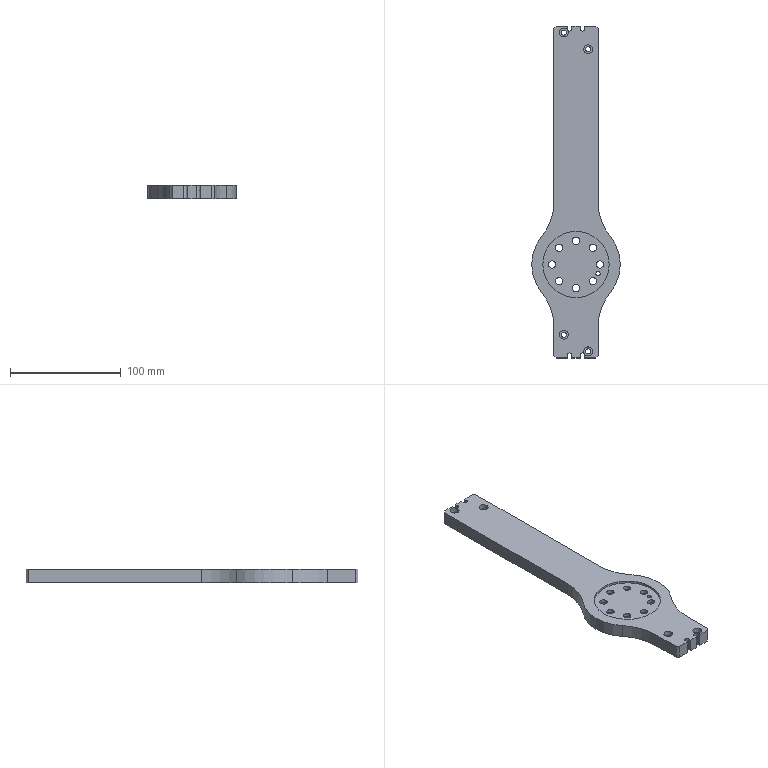Part | SolidWorks | features Cut 3, HoleWzd 3, Chamfer 2, CirPattern 1, Extrusion 1, Fillet 1 | 1 solid | 100 faces | box 80 x 300 x 12 mm | volume 155894 mm3 | cylinder 63 | plane 37 | commonest cylinder face diameters 6.6 x16 11 x16 4.5 x8 8 x8 4.2 x4 100 x4